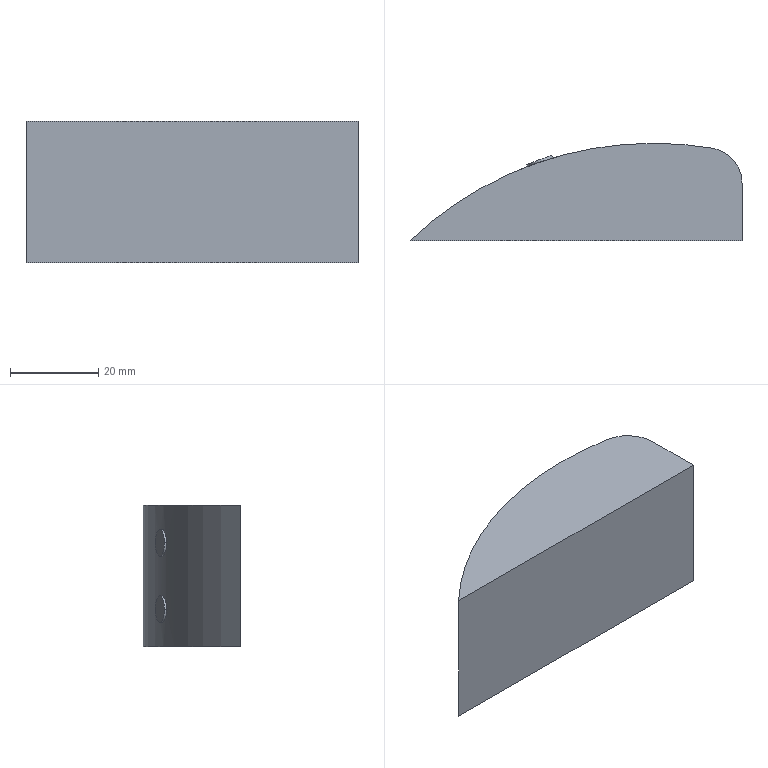Part | STEP file | _CKZT-T040.stp | 1 solid | 12 faces | box 75.1 x 22 x 32 mm | volume 39956 mm3 | plane 6 | cylinder 6 | commonest cylinder face diameters 6 x4 16 x1 160 x1